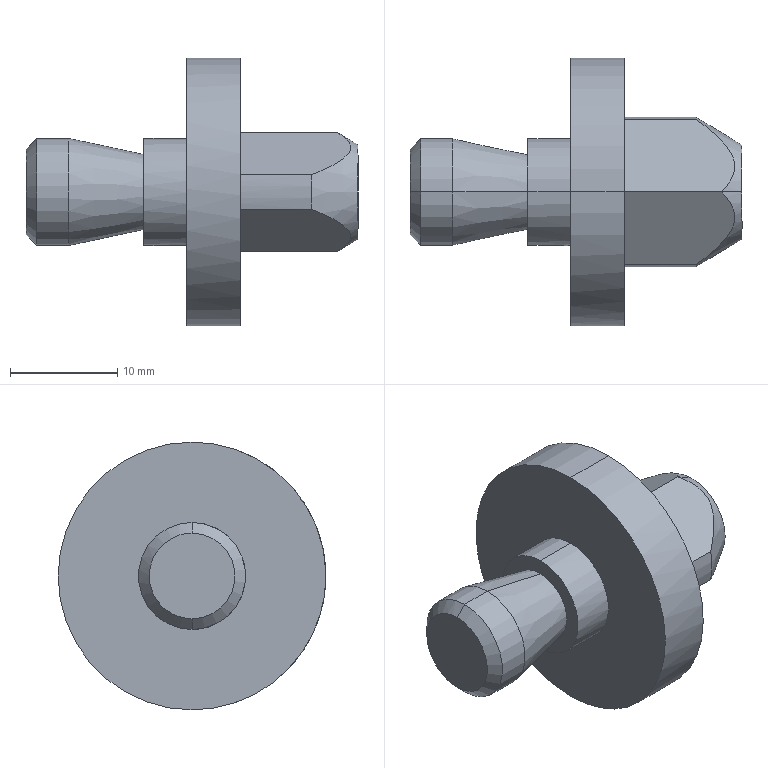Part | STEP file | Positioning_id1790_x_t | 1 solid | 23 faces | box 31 x 25 x 25 mm | volume 4491 mm3 | plane 9 | cylinder 8 | cone 6 | commonest cylinder face diameters 10 x4 14 x2 25 x2